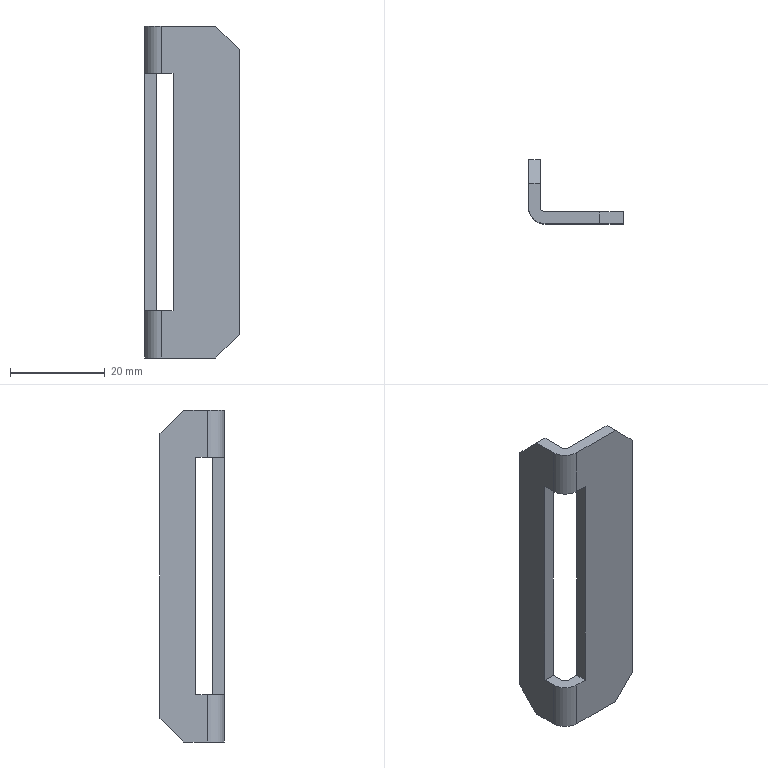Part | STEP file | AP0_JYDM_SHEET_15 | 1 solid | 20 faces | box 20 x 13.5 x 70 mm | volume 4064 mm3 | plane 16 | cylinder 4 | commonest cylinder face diameters 2 x2 7 x2
STEP:
#1=CARTESIAN_POINT('',(6.,2.5,25.));
#2=VERTEX_POINT('',#1);
#3=CARTESIAN_POINT('',(6.,2.5,-25.));
#4=VERTEX_POINT('',#3);
#5=CARTESIAN_POINT('',(6.,2.5,-35.));
#6=DIRECTION('',(0.,0.,-1.));
#7=VECTOR('',#6,1000.);
#8=LINE('',#5,#7);
#9=EDGE_CURVE('',#2,#4,#8,.T.);
#10=ORIENTED_EDGE('',*,*,#9,.F.);
#11=CARTESIAN_POINT('',(3.5,2.5,25.));
#12=VERTEX_POINT('',#11);
#13=CARTESIAN_POINT('',(0.,2.5,25.));
#14=DIRECTION('',(1.,0.,0.));
#15=VECTOR('',#14,1000.);
#16=LINE('',#13,#15);
#17=EDGE_CURVE('',#12,#2,#16,.T.);
#18=ORIENTED_EDGE('',*,*,#17,.F.);
#19=CARTESIAN_POINT('',(3.5,2.5,35.));
#20=VERTEX_POINT('',#19);
#21=CARTESIAN_POINT('',(3.5,2.5,-35.));
#22=DIRECTION('',(0.,0.,-1.));
#23=VECTOR('',#22,1000.);
#24=LINE('',#21,#23);
#25=EDGE_CURVE('',#20,#12,#24,.T.);
#26=ORIENTED_EDGE('',*,*,#25,.F.);
#27=CARTESIAN_POINT('',(15.,2.5,35.));
#28=VERTEX_POINT('',#27);
#29=CARTESIAN_POINT('',(0.,2.5,35.));
#30=DIRECTION('',(-1.,0.,0.));
#31=VECTOR('',#30,1000.);
#32=LINE('',#29,#31);
#33=EDGE_CURVE('',#28,#20,#32,.T.);
#34=ORIENTED_EDGE('',*,*,#33,.F.);
#35=CARTESIAN_POINT('',(20.,2.5,30.));
#36=VERTEX_POINT('',#35);
#37=CARTESIAN_POINT('',(20.,2.5,30.));
#38=DIRECTION('',(-0.7071,0.,0.7071));
#39=VECTOR('',#38,1000.);
#40=LINE('',#37,#39);
#41=EDGE_CURVE('',#36,#28,#40,.T.);
#42=ORIENTED_EDGE('',*,*,#41,.F.);
#43=CARTESIAN_POINT('',(20.,2.5,-30.));
#44=VERTEX_POINT('',#43);
#45=CARTESIAN_POINT('',(20.,2.5,-35.));
#46=DIRECTION('',(0.,0.,1.));
#47=VECTOR('',#46,1000.);
#48=LINE('',#45,#47);
#49=EDGE_CURVE('',#44,#36,#48,.T.);
#50=ORIENTED_EDGE('',*,*,#49,.F.);
#51=CARTESIAN_POINT('',(15.,2.5,-35.));
#52=VERTEX_POINT('',#51);
#53=CARTESIAN_POINT('',(15.,2.5,-35.));
#54=DIRECTION('',(0.7071,0.,0.7071));
#55=VECTOR('',#54,1000.);
#56=LINE('',#53,#55);
#57=EDGE_CURVE('',#52,#44,#56,.T.);
#58=ORIENTED_EDGE('',*,*,#57,.F.);
#59=CARTESIAN_POINT('',(3.5,2.5,-35.));
#60=VERTEX_POINT('',#59);
#61=CARTESIAN_POINT('',(0.,2.5,-35.));
#62=DIRECTION('',(1.,0.,0.));
#63=VECTOR('',#62,1000.);
#64=LINE('',#61,#63);
#65=EDGE_CURVE('',#60,#52,#64,.T.);
#66=ORIENTED_EDGE('',*,*,#65,.F.);
#67=CARTESIAN_POINT('',(3.5,2.5,-25.));
#68=VERTEX_POINT('',#67);
#69=CARTESIAN_POINT('',(3.5,2.5,-35.));
#70=DIRECTION('',(0.,0.,-1.));
#71=VECTOR('',#70,1000.);
#72=LINE('',#69,#71);
#73=EDGE_CURVE('',#68,#60,#72,.T.);
#74=ORIENTED_EDGE('',*,*,#73,.F.);
#75=CARTESIAN_POINT('',(0.,2.5,-25.));
#76=DIRECTION('',(-1.,0.,0.));
#77=VECTOR('',#76,1000.);
#78=LINE('',#75,#77);
#79=EDGE_CURVE('',#4,#68,#78,.T.);
#80=ORIENTED_EDGE('',*,*,#79,.F.);
#81=EDGE_LOOP('',(#10,#18,#26,#34,#42,#50,#58,#66,#74,#80));
#82=FACE_OUTER_BOUND('',#81,.T.);
#83=CARTESIAN_POINT('',(0.,2.5,-35.));
#84=DIRECTION('',(0.,-1.,0.));
#85=DIRECTION('',(0.,0.,-1.));
#86=AXIS2_PLACEMENT_3D('',#83,#84,#85);
#87=PLANE('',#86);
#88=ADVANCED_FACE('',(#82),#87,.F.);
#89=CARTESIAN_POINT('',(2.5,6.,-25.));
#90=VERTEX_POINT('',#89);
#91=CARTESIAN_POINT('',(2.5,3.5,-25.));
#92=VERTEX_POINT('',#91);
#93=CARTESIAN_POINT('',(2.5,1.25,-25.));
#94=DIRECTION('',(0.,-1.,0.));
#95=VECTOR('',#94,1000.);
#96=LINE('',#93,#95);
#97=EDGE_CURVE('',#90,#92,#96,.T.);
#98=ORIENTED_EDGE('',*,*,#97,.F.);
#99=CARTESIAN_POINT('',(0.,6.,-25.));
#100=VERTEX_POINT('',#99);
#101=CARTESIAN_POINT('',(4.75,6.,-25.));
#102=DIRECTION('',(1.,0.,0.));
#103=VECTOR('',#102,1000.);
#104=LINE('',#101,#103);
#105=EDGE_CURVE('',#100,#90,#104,.T.);
#106=ORIENTED_EDGE('',*,*,#105,.F.);
#107=CARTESIAN_POINT('',(0.,3.5,-25.));
#108=VERTEX_POINT('',#107);
#109=CARTESIAN_POINT('',(0.,1.25,-25.));
#110=DIRECTION('',(0.,1.,0.));
#111=VECTOR('',#110,1000.);
#112=LINE('',#109,#111);
#113=EDGE_CURVE('',#108,#100,#112,.T.);
#114=ORIENTED_EDGE('',*,*,#113,.F.);
#115=CARTESIAN_POINT('',(3.5,0.,-25.));
#116=VERTEX_POINT('',#115);
#117=CARTESIAN_POINT('',(3.5,3.5,-25.));
#118=DIRECTION('',(0.,0.,-1.));
#119=DIRECTION('',(-1.,0.,0.));
#120=AXIS2_PLACEMENT_3D('',#117,#118,#119);
#121=CIRCLE('',#120,3.5);
#122=EDGE_CURVE('',#116,#108,#121,.T.);
#123=ORIENTED_EDGE('',*,*,#122,.F.);
#124=CARTESIAN_POINT('',(6.,0.,-25.));
#125=VERTEX_POINT('',#124);
#126=CARTESIAN_POINT('',(4.75,0.,-25.));
#127=DIRECTION('',(-1.,0.,0.));
#128=VECTOR('',#127,1000.);
#129=LINE('',#126,#128);
#130=EDGE_CURVE('',#125,#116,#129,.T.);
#131=ORIENTED_EDGE('',*,*,#130,.F.);
#132=CARTESIAN_POINT('',(6.,1.25,-25.));
#133=DIRECTION('',(0.,-1.,0.));
#134=VECTOR('',#133,1000.);
#135=LINE('',#132,#134);
#136=EDGE_CURVE('',#4,#125,#135,.T.);
#137=ORIENTED_EDGE('',*,*,#136,.F.);
#138=ORIENTED_EDGE('',*,*,#79,.T.);
#139=CARTESIAN_POINT('',(3.5,3.5,-25.));
#140=DIRECTION('',(0.,0.,1.));
#141=DIRECTION('',(-1.,0.,0.));
#142=AXIS2_PLACEMENT_3D('',#139,#140,#141);
#143=CIRCLE('',#142,1.);
#144=EDGE_CURVE('',#92,#68,#143,.T.);
#145=ORIENTED_EDGE('',*,*,#144,.F.);
#146=EDGE_LOOP('',(#98,#106,#114,#123,#131,#137,#138,#145));
#147=FACE_OUTER_BOUND('',#146,.T.);
#148=CARTESIAN_POINT('',(4.75,1.25,-25.));
#149=DIRECTION('',(0.,0.,-1.));
#150=DIRECTION('',(-1.,0.,0.));
#151=AXIS2_PLACEMENT_3D('',#148,#149,#150);
#152=PLANE('',#151);
#153=ADVANCED_FACE('',(#147),#152,.F.);
#154=CARTESIAN_POINT('',(6.,0.,25.));
#155=VERTEX_POINT('',#154);
#156=CARTESIAN_POINT('',(6.,0.,0.));
#157=DIRECTION('',(0.,0.,-1.));
#158=VECTOR('',#157,1000.);
#159=LINE('',#156,#158);
#160=EDGE_CURVE('',#155,#125,#159,.T.);
#161=ORIENTED_EDGE('',*,*,#160,.F.);
#162=CARTESIAN_POINT('',(6.,1.25,25.));
#163=DIRECTION('',(0.,-1.,0.));
#164=VECTOR('',#163,1000.);
#165=LINE('',#162,#164);
#166=EDGE_CURVE('',#2,#155,#165,.T.);
#167=ORIENTED_EDGE('',*,*,#166,.F.);
#168=ORIENTED_EDGE('',*,*,#9,.T.);
#169=ORIENTED_EDGE('',*,*,#136,.T.);
#170=EDGE_LOOP('',(#161,#167,#168,#169));
#171=FACE_OUTER_BOUND('',#170,.T.);
#172=CARTESIAN_POINT('',(6.,1.25,0.));
#173=DIRECTION('',(1.,0.,0.));
#174=DIRECTION('',(0.,0.,-1.));
#175=AXIS2_PLACEMENT_3D('',#172,#173,#174);
#176=PLANE('',#175);
#177=ADVANCED_FACE('',(#171),#176,.F.);
#178=CARTESIAN_POINT('',(0.,6.,25.));
#179=VERTEX_POINT('',#178);
#180=CARTESIAN_POINT('',(2.5,6.,25.));
#181=VERTEX_POINT('',#180);
#182=CARTESIAN_POINT('',(4.75,6.,25.));
#183=DIRECTION('',(1.,0.,0.));
#184=VECTOR('',#183,1000.);
#185=LINE('',#182,#184);
#186=EDGE_CURVE('',#179,#181,#185,.T.);
#187=ORIENTED_EDGE('',*,*,#186,.T.);
#188=CARTESIAN_POINT('',(2.5,3.5,25.));
#189=VERTEX_POINT('',#188);
#190=CARTESIAN_POINT('',(2.5,1.25,25.));
#191=DIRECTION('',(0.,-1.,0.));
#192=VECTOR('',#191,1000.);
#193=LINE('',#190,#192);
#194=EDGE_CURVE('',#181,#189,#193,.T.);
#195=ORIENTED_EDGE('',*,*,#194,.T.);
#196=CARTESIAN_POINT('',(3.5,3.5,25.));
#197=DIRECTION('',(0.,0.,1.));
#198=DIRECTION('',(-1.,0.,0.));
#199=AXIS2_PLACEMENT_3D('',#196,#197,#198);
#200=CIRCLE('',#199,1.);
#201=EDGE_CURVE('',#189,#12,#200,.T.);
#202=ORIENTED_EDGE('',*,*,#201,.T.);
#203=ORIENTED_EDGE('',*,*,#17,.T.);
#204=ORIENTED_EDGE('',*,*,#166,.T.);
#205=CARTESIAN_POINT('',(3.5,0.,25.));
#206=VERTEX_POINT('',#205);
#207=CARTESIAN_POINT('',(4.75,0.,25.));
#208=DIRECTION('',(-1.,0.,0.));
#209=VECTOR('',#208,1000.);
#210=LINE('',#207,#209);
#211=EDGE_CURVE('',#155,#206,#210,.T.);
#212=ORIENTED_EDGE('',*,*,#211,.T.);
#213=CARTESIAN_POINT('',(0.,3.5,25.));
#214=VERTEX_POINT('',#213);
#215=CARTESIAN_POINT('',(3.5,3.5,25.));
#216=DIRECTION('',(0.,0.,-1.));
#217=DIRECTION('',(-1.,0.,0.));
#218=AXIS2_PLACEMENT_3D('',#215,#216,#217);
#219=CIRCLE('',#218,3.5);
#220=EDGE_CURVE('',#206,#214,#219,.T.);
#221=ORIENTED_EDGE('',*,*,#220,.T.);
#222=CARTESIAN_POINT('',(0.,1.25,25.));
#223=DIRECTION('',(0.,1.,0.));
#224=VECTOR('',#223,1000.);
#225=LINE('',#222,#224);
#226=EDGE_CURVE('',#214,#179,#225,.T.);
#227=ORIENTED_EDGE('',*,*,#226,.T.);
#228=EDGE_LOOP('',(#187,#195,#202,#203,#204,#212,#221,#227));
#229=FACE_OUTER_BOUND('',#228,.T.);
#230=CARTESIAN_POINT('',(4.75,1.25,25.));
#231=DIRECTION('',(0.,0.,-1.));
#232=DIRECTION('',(-1.,0.,0.));
#233=AXIS2_PLACEMENT_3D('',#230,#231,#232);
#234=PLANE('',#233);
#235=ADVANCED_FACE('',(#229),#234,.T.);
#236=ORIENTED_EDGE('',*,*,#201,.F.);
#237=CARTESIAN_POINT('',(2.5,3.5,35.));
#238=VERTEX_POINT('',#237);
#239=CARTESIAN_POINT('',(2.5,3.5,-35.));
#240=DIRECTION('',(0.,0.,-1.));
#241=VECTOR('',#240,1000.);
#242=LINE('',#239,#241);
#243=EDGE_CURVE('',#238,#189,#242,.T.);
#244=ORIENTED_EDGE('',*,*,#243,.F.);
#245=CARTESIAN_POINT('',(3.5,3.5,35.));
#246=DIRECTION('',(0.,0.,-1.));
#247=DIRECTION('',(-1.,0.,0.));
#248=AXIS2_PLACEMENT_3D('',#245,#246,#247);
#249=CIRCLE('',#248,1.);
#250=EDGE_CURVE('',#20,#238,#249,.T.);
#251=ORIENTED_EDGE('',*,*,#250,.F.);
#252=ORIENTED_EDGE('',*,*,#25,.T.);
#253=EDGE_LOOP('',(#236,#244,#251,#252));
#254=FACE_OUTER_BOUND('',#253,.T.);
#255=CARTESIAN_POINT('',(3.5,3.5,-35.));
#256=DIRECTION('',(0.,0.,-1.));
#257=DIRECTION('',(-1.,0.,0.));
#258=AXIS2_PLACEMENT_3D('',#255,#256,#257);
#259=CYLINDRICAL_SURFACE('',#258,1.);
#260=ADVANCED_FACE('',(#254),#259,.F.);
#261=CARTESIAN_POINT('',(2.5,8.5,35.));
#262=VERTEX_POINT('',#261);
#263=CARTESIAN_POINT('',(2.5,1.25,35.));
#264=DIRECTION('',(0.,-1.,0.));
#265=VECTOR('',#264,1000.);
#266=LINE('',#263,#265);
#267=EDGE_CURVE('',#262,#238,#266,.T.);
#268=ORIENTED_EDGE('',*,*,#267,.F.);
#269=CARTESIAN_POINT('',(0.,8.5,35.));
#270=VERTEX_POINT('',#269);
#271=CARTESIAN_POINT('',(11.75,8.5,35.));
#272=DIRECTION('',(1.,0.,0.));
#273=VECTOR('',#272,1000.);
#274=LINE('',#271,#273);
#275=EDGE_CURVE('',#270,#262,#274,.T.);
#276=ORIENTED_EDGE('',*,*,#275,.F.);
#277=CARTESIAN_POINT('',(0.,3.5,35.));
#278=VERTEX_POINT('',#277);
#279=CARTESIAN_POINT('',(0.,1.25,35.));
#280=DIRECTION('',(0.,1.,0.));
#281=VECTOR('',#280,1000.);
#282=LINE('',#279,#281);
#283=EDGE_CURVE('',#278,#270,#282,.T.);
#284=ORIENTED_EDGE('',*,*,#283,.F.);
#285=CARTESIAN_POINT('',(3.5,0.,35.));
#286=VERTEX_POINT('',#285);
#287=CARTESIAN_POINT('',(3.5,3.5,35.));
#288=DIRECTION('',(0.,0.,-1.));
#289=DIRECTION('',(-1.,0.,0.));
#290=AXIS2_PLACEMENT_3D('',#287,#288,#289);
#291=CIRCLE('',#290,3.5);
#292=EDGE_CURVE('',#286,#278,#291,.T.);
#293=ORIENTED_EDGE('',*,*,#292,.F.);
#294=CARTESIAN_POINT('',(15.,0.,35.));
#295=VERTEX_POINT('',#294);
#296=CARTESIAN_POINT('',(11.75,0.,35.));
#297=DIRECTION('',(-1.,0.,0.));
#298=VECTOR('',#297,1000.);
#299=LINE('',#296,#298);
#300=EDGE_CURVE('',#295,#286,#299,.T.);
#301=ORIENTED_EDGE('',*,*,#300,.F.);
#302=CARTESIAN_POINT('',(15.,1.25,35.));
#303=DIRECTION('',(0.,-1.,0.));
#304=VECTOR('',#303,1000.);
#305=LINE('',#302,#304);
#306=EDGE_CURVE('',#28,#295,#305,.T.);
#307=ORIENTED_EDGE('',*,*,#306,.F.);
#308=ORIENTED_EDGE('',*,*,#33,.T.);
#309=ORIENTED_EDGE('',*,*,#250,.T.);
#310=EDGE_LOOP('',(#268,#276,#284,#293,#301,#307,#308,#309));
#311=FACE_OUTER_BOUND('',#310,.T.);
#312=CARTESIAN_POINT('',(11.75,1.25,35.));
#313=DIRECTION('',(0.,0.,-1.));
#314=DIRECTION('',(-1.,0.,0.));
#315=AXIS2_PLACEMENT_3D('',#312,#313,#314);
#316=PLANE('',#315);
#317=ADVANCED_FACE('',(#311),#316,.F.);
#318=ORIENTED_EDGE('',*,*,#306,.T.);
#319=CARTESIAN_POINT('',(20.,0.,30.));
#320=VERTEX_POINT('',#319);
#321=CARTESIAN_POINT('',(17.5,0.,32.5));
#322=DIRECTION('',(0.7071,0.,-0.7071));
#323=VECTOR('',#322,1000.);
#324=LINE('',#321,#323);
#325=EDGE_CURVE('',#295,#320,#324,.T.);
#326=ORIENTED_EDGE('',*,*,#325,.T.);
#327=CARTESIAN_POINT('',(20.,1.25,30.));
#328=DIRECTION('',(0.,1.,0.));
#329=VECTOR('',#328,1000.);
#330=LINE('',#327,#329);
#331=EDGE_CURVE('',#320,#36,#330,.T.);
#332=ORIENTED_EDGE('',*,*,#331,.T.);
#333=ORIENTED_EDGE('',*,*,#41,.T.);
#334=EDGE_LOOP('',(#318,#326,#332,#333));
#335=FACE_OUTER_BOUND('',#334,.T.);
#336=CARTESIAN_POINT('',(17.5,1.25,32.5));
#337=DIRECTION('',(0.7071,0.,0.7071));
#338=DIRECTION('',(0.7071,0.,-0.7071));
#339=AXIS2_PLACEMENT_3D('',#336,#337,#338);
#340=PLANE('',#339);
#341=ADVANCED_FACE('',(#335),#340,.T.);
#342=CARTESIAN_POINT('',(20.,0.,-30.));
#343=VERTEX_POINT('',#342);
#344=CARTESIAN_POINT('',(20.,0.,0.));
#345=DIRECTION('',(0.,0.,-1.));
#346=VECTOR('',#345,1000.);
#347=LINE('',#344,#346);
#348=EDGE_CURVE('',#320,#343,#347,.T.);
#349=ORIENTED_EDGE('',*,*,#348,.T.);
#350=CARTESIAN_POINT('',(20.,1.25,-30.));
#351=DIRECTION('',(0.,1.,0.));
#352=VECTOR('',#351,1000.);
#353=LINE('',#350,#352);
#354=EDGE_CURVE('',#343,#44,#353,.T.);
#355=ORIENTED_EDGE('',*,*,#354,.T.);
#356=ORIENTED_EDGE('',*,*,#49,.T.);
#357=ORIENTED_EDGE('',*,*,#331,.F.);
#358=EDGE_LOOP('',(#349,#355,#356,#357));
#359=FACE_OUTER_BOUND('',#358,.T.);
#360=CARTESIAN_POINT('',(20.,1.25,0.));
#361=DIRECTION('',(1.,0.,0.));
#362=DIRECTION('',(0.,0.,-1.));
#363=AXIS2_PLACEMENT_3D('',#360,#361,#362);
#364=PLANE('',#363);
#365=ADVANCED_FACE('',(#359),#364,.T.);
#366=ORIENTED_EDGE('',*,*,#354,.F.);
#367=CARTESIAN_POINT('',(15.,0.,-35.));
#368=VERTEX_POINT('',#367);
#369=CARTESIAN_POINT('',(17.5,0.,-32.5));
#370=DIRECTION('',(-0.7071,0.,-0.7071));
#371=VECTOR('',#370,1000.);
#372=LINE('',#369,#371);
#373=EDGE_CURVE('',#343,#368,#372,.T.);
#374=ORIENTED_EDGE('',*,*,#373,.T.);
#375=CARTESIAN_POINT('',(15.,1.25,-35.));
#376=DIRECTION('',(0.,1.,0.));
#377=VECTOR('',#376,1000.);
#378=LINE('',#375,#377);
#379=EDGE_CURVE('',#368,#52,#378,.T.);
#380=ORIENTED_EDGE('',*,*,#379,.T.);
#381=ORIENTED_EDGE('',*,*,#57,.T.);
#382=EDGE_LOOP('',(#366,#374,#380,#381));
#383=FACE_OUTER_BOUND('',#382,.T.);
#384=CARTESIAN_POINT('',(17.5,1.25,-32.5));
#385=DIRECTION('',(0.7071,0.,-0.7071));
#386=DIRECTION('',(-0.7071,0.,-0.7071));
#387=AXIS2_PLACEMENT_3D('',#384,#385,#386);
#388=PLANE('',#387);
#389=ADVANCED_FACE('',(#383),#388,.T.);
#390=CARTESIAN_POINT('',(0.,3.5,-35.));
#391=VERTEX_POINT('',#390);
#392=CARTESIAN_POINT('',(0.,8.5,-35.));
#393=VERTEX_POINT('',#392);
#394=CARTESIAN_POINT('',(0.,1.25,-35.));
#395=DIRECTION('',(0.,1.,0.));
#396=VECTOR('',#395,1000.);
#397=LINE('',#394,#396);
#398=EDGE_CURVE('',#391,#393,#397,.T.);
#399=ORIENTED_EDGE('',*,*,#398,.T.);
#400=CARTESIAN_POINT('',(2.5,8.5,-35.));
#401=VERTEX_POINT('',#400);
#402=CARTESIAN_POINT('',(11.75,8.5,-35.));
#403=DIRECTION('',(1.,0.,0.));
#404=VECTOR('',#403,1000.);
#405=LINE('',#402,#404);
#406=EDGE_CURVE('',#393,#401,#405,.T.);
#407=ORIENTED_EDGE('',*,*,#406,.T.);
#408=CARTESIAN_POINT('',(2.5,3.5,-35.));
#409=VERTEX_POINT('',#408);
#410=CARTESIAN_POINT('',(2.5,1.25,-35.));
#411=DIRECTION('',(0.,-1.,0.));
#412=VECTOR('',#411,1000.);
#413=LINE('',#410,#412);
#414=EDGE_CURVE('',#401,#409,#413,.T.);
#415=ORIENTED_EDGE('',*,*,#414,.T.);
#416=CARTESIAN_POINT('',(3.5,3.5,-35.));
#417=DIRECTION('',(0.,0.,1.));
#418=DIRECTION('',(-1.,0.,0.));
#419=AXIS2_PLACEMENT_3D('',#416,#417,#418);
#420=CIRCLE('',#419,1.);
#421=EDGE_CURVE('',#409,#60,#420,.T.);
#422=ORIENTED_EDGE('',*,*,#421,.T.);
#423=ORIENTED_EDGE('',*,*,#65,.T.);
#424=ORIENTED_EDGE('',*,*,#379,.F.);
#425=CARTESIAN_POINT('',(3.5,0.,-35.));
#426=VERTEX_POINT('',#425);
#427=CARTESIAN_POINT('',(11.75,0.,-35.));
#428=DIRECTION('',(-1.,0.,0.));
#429=VECTOR('',#428,1000.);
#430=LINE('',#427,#429);
#431=EDGE_CURVE('',#368,#426,#430,.T.);
#432=ORIENTED_EDGE('',*,*,#431,.T.);
#433=CARTESIAN_POINT('',(3.5,3.5,-35.));
#434=DIRECTION('',(0.,0.,-1.));
#435=DIRECTION('',(-1.,0.,0.));
#436=AXIS2_PLACEMENT_3D('',#433,#434,#435);
#437=CIRCLE('',#436,3.5);
#438=EDGE_CURVE('',#426,#391,#437,.T.);
#439=ORIENTED_EDGE('',*,*,#438,.T.);
#440=EDGE_LOOP('',(#399,#407,#415,#422,#423,#424,#432,#439));
#441=FACE_OUTER_BOUND('',#440,.T.);
#442=CARTESIAN_POINT('',(11.75,1.25,-35.));
#443=DIRECTION('',(0.,0.,-1.));
#444=DIRECTION('',(-1.,0.,0.));
#445=AXIS2_PLACEMENT_3D('',#442,#443,#444);
#446=PLANE('',#445);
#447=ADVANCED_FACE('',(#441),#446,.T.);
#448=ORIENTED_EDGE('',*,*,#144,.T.);
#449=ORIENTED_EDGE('',*,*,#73,.T.);
#450=ORIENTED_EDGE('',*,*,#421,.F.);
#451=CARTESIAN_POINT('',(2.5,3.5,-35.));
#452=DIRECTION('',(0.,0.,-1.));
#453=VECTOR('',#452,1000.);
#454=LINE('',#451,#453);
#455=EDGE_CURVE('',#92,#409,#454,.T.);
#456=ORIENTED_EDGE('',*,*,#455,.F.);
#457=EDGE_LOOP('',(#448,#449,#450,#456));
#458=FACE_OUTER_BOUND('',#457,.T.);
#459=CARTESIAN_POINT('',(3.5,3.5,-35.));
#460=DIRECTION('',(0.,0.,-1.));
#461=DIRECTION('',(-1.,0.,0.));
#462=AXIS2_PLACEMENT_3D('',#459,#460,#461);
#463=CYLINDRICAL_SURFACE('',#462,1.);
#464=ADVANCED_FACE('',(#458),#463,.F.);
#465=CARTESIAN_POINT('',(2.5,6.,-35.));
#466=DIRECTION('',(0.,0.,1.));
#467=VECTOR('',#466,1000.);
#468=LINE('',#465,#467);
#469=EDGE_CURVE('',#90,#181,#468,.T.);
#470=ORIENTED_EDGE('',*,*,#469,.F.);
#471=ORIENTED_EDGE('',*,*,#97,.T.);
#472=ORIENTED_EDGE('',*,*,#455,.T.);
#473=ORIENTED_EDGE('',*,*,#414,.F.);
#474=CARTESIAN_POINT('',(2.5,13.5,-30.));
#475=VERTEX_POINT('',#474);
#476=CARTESIAN_POINT('',(2.5,13.5,-30.));
#477=DIRECTION('',(0.,-0.7071,-0.7071));
#478=VECTOR('',#477,1000.);
#479=LINE('',#476,#478);
#480=EDGE_CURVE('',#475,#401,#479,.T.);
#481=ORIENTED_EDGE('',*,*,#480,.F.);
#482=CARTESIAN_POINT('',(2.5,13.5,30.));
#483=VERTEX_POINT('',#482);
#484=CARTESIAN_POINT('',(2.5,13.5,-35.));
#485=DIRECTION('',(0.,0.,-1.));
#486=VECTOR('',#485,1000.);
#487=LINE('',#484,#486);
#488=EDGE_CURVE('',#483,#475,#487,.T.);
#489=ORIENTED_EDGE('',*,*,#488,.F.);
#490=CARTESIAN_POINT('',(2.5,8.5,35.));
#491=DIRECTION('',(0.,0.7071,-0.7071));
#492=VECTOR('',#491,1000.);
#493=LINE('',#490,#492);
#494=EDGE_CURVE('',#262,#483,#493,.T.);
#495=ORIENTED_EDGE('',*,*,#494,.F.);
#496=ORIENTED_EDGE('',*,*,#267,.T.);
#497=ORIENTED_EDGE('',*,*,#243,.T.);
#498=ORIENTED_EDGE('',*,*,#194,.F.);
#499=EDGE_LOOP('',(#470,#471,#472,#473,#481,#489,#495,#496,#497,#498));
#500=FACE_OUTER_BOUND('',#499,.T.);
#501=CARTESIAN_POINT('',(2.5,13.5,-35.));
#502=DIRECTION('',(-1.,0.,0.));
#503=DIRECTION('',(0.,0.,1.));
#504=AXIS2_PLACEMENT_3D('',#501,#502,#503);
#505=PLANE('',#504);
#506=ADVANCED_FACE('',(#500),#505,.F.);
#507=ORIENTED_EDGE('',*,*,#186,.F.);
#508=CARTESIAN_POINT('',(0.,6.,0.));
#509=DIRECTION('',(0.,0.,-1.));
#510=VECTOR('',#509,1000.);
#511=LINE('',#508,#510);
#512=EDGE_CURVE('',#179,#100,#511,.T.);
#513=ORIENTED_EDGE('',*,*,#512,.T.);
#514=ORIENTED_EDGE('',*,*,#105,.T.);
#515=ORIENTED_EDGE('',*,*,#469,.T.);
#516=EDGE_LOOP('',(#507,#513,#514,#515));
#517=FACE_OUTER_BOUND('',#516,.T.);
#518=CARTESIAN_POINT('',(1.25,6.,0.));
#519=DIRECTION('',(0.,-1.,0.));
#520=DIRECTION('',(0.,0.,-1.));
#521=AXIS2_PLACEMENT_3D('',#518,#519,#520);
#522=PLANE('',#521);
#523=ADVANCED_FACE('',(#517),#522,.T.);
#524=ORIENTED_EDGE('',*,*,#113,.T.);
#525=ORIENTED_EDGE('',*,*,#512,.F.);
#526=ORIENTED_EDGE('',*,*,#226,.F.);
#527=CARTESIAN_POINT('',(0.,3.5,-35.));
#528=DIRECTION('',(0.,0.,1.));
#529=VECTOR('',#528,1000.);
#530=LINE('',#527,#529);
#531=EDGE_CURVE('',#214,#278,#530,.T.);
#532=ORIENTED_EDGE('',*,*,#531,.T.);
#533=ORIENTED_EDGE('',*,*,#283,.T.);
#534=CARTESIAN_POINT('',(0.,13.5,30.));
#535=VERTEX_POINT('',#534);
#536=CARTESIAN_POINT('',(0.,8.5,35.));
#537=DIRECTION('',(0.,0.7071,-0.7071));
#538=VECTOR('',#537,1000.);
#539=LINE('',#536,#538);
#540=EDGE_CURVE('',#270,#535,#539,.T.);
#541=ORIENTED_EDGE('',*,*,#540,.T.);
#542=CARTESIAN_POINT('',(0.,13.5,-30.));
#543=VERTEX_POINT('',#542);
#544=CARTESIAN_POINT('',(0.,13.5,-35.));
#545=DIRECTION('',(0.,0.,-1.));
#546=VECTOR('',#545,1000.);
#547=LINE('',#544,#546);
#548=EDGE_CURVE('',#535,#543,#547,.T.);
#549=ORIENTED_EDGE('',*,*,#548,.T.);
#550=CARTESIAN_POINT('',(0.,13.5,-30.));
#551=DIRECTION('',(0.,-0.7071,-0.7071));
#552=VECTOR('',#551,1000.);
#553=LINE('',#550,#552);
#554=EDGE_CURVE('',#543,#393,#553,.T.);
#555=ORIENTED_EDGE('',*,*,#554,.T.);
#556=ORIENTED_EDGE('',*,*,#398,.F.);
#557=CARTESIAN_POINT('',(0.,3.5,-35.));
#558=DIRECTION('',(0.,0.,1.));
#559=VECTOR('',#558,1000.);
#560=LINE('',#557,#559);
#561=EDGE_CURVE('',#391,#108,#560,.T.);
#562=ORIENTED_EDGE('',*,*,#561,.T.);
#563=EDGE_LOOP('',(#524,#525,#526,#532,#533,#541,#549,#555,#556,#562));
#564=FACE_OUTER_BOUND('',#563,.T.);
#565=CARTESIAN_POINT('',(0.,13.5,-35.));
#566=DIRECTION('',(-1.,0.,0.));
#567=DIRECTION('',(0.,0.,1.));
#568=AXIS2_PLACEMENT_3D('',#565,#566,#567);
#569=PLANE('',#568);
#570=ADVANCED_FACE('',(#564),#569,.T.);
#571=CARTESIAN_POINT('',(3.5,0.,-35.));
#572=DIRECTION('',(0.,0.,1.));
#573=VECTOR('',#572,1000.);
#574=LINE('',#571,#573);
#575=EDGE_CURVE('',#426,#116,#574,.T.);
#576=ORIENTED_EDGE('',*,*,#575,.T.);
#577=ORIENTED_EDGE('',*,*,#122,.T.);
#578=ORIENTED_EDGE('',*,*,#561,.F.);
#579=ORIENTED_EDGE('',*,*,#438,.F.);
#580=EDGE_LOOP('',(#576,#577,#578,#579));
#581=FACE_OUTER_BOUND('',#580,.T.);
#582=CARTESIAN_POINT('',(3.5,3.5,-35.));
#583=DIRECTION('',(0.,0.,-1.));
#584=DIRECTION('',(-1.,0.,0.));
#585=AXIS2_PLACEMENT_3D('',#582,#583,#584);
#586=CYLINDRICAL_SURFACE('',#585,3.5);
#587=ADVANCED_FACE('',(#581),#586,.T.);
#588=ORIENTED_EDGE('',*,*,#211,.F.);
#589=ORIENTED_EDGE('',*,*,#160,.T.);
#590=ORIENTED_EDGE('',*,*,#130,.T.);
#591=ORIENTED_EDGE('',*,*,#575,.F.);
#592=ORIENTED_EDGE('',*,*,#431,.F.);
#593=ORIENTED_EDGE('',*,*,#373,.F.);
#594=ORIENTED_EDGE('',*,*,#348,.F.);
#595=ORIENTED_EDGE('',*,*,#325,.F.);
#596=ORIENTED_EDGE('',*,*,#300,.T.);
#597=CARTESIAN_POINT('',(3.5,0.,-35.));
#598=DIRECTION('',(0.,0.,-1.));
#599=VECTOR('',#598,1000.);
#600=LINE('',#597,#599);
#601=EDGE_CURVE('',#286,#206,#600,.T.);
#602=ORIENTED_EDGE('',*,*,#601,.T.);
#603=EDGE_LOOP('',(#588,#589,#590,#591,#592,#593,#594,#595,#596,#602));
#604=FACE_OUTER_BOUND('',#603,.T.);
#605=CARTESIAN_POINT('',(0.,0.,-35.));
#606=DIRECTION('',(0.,-1.,0.));
#607=DIRECTION('',(0.,0.,-1.));
#608=AXIS2_PLACEMENT_3D('',#605,#606,#607);
#609=PLANE('',#608);
#610=ADVANCED_FACE('',(#604),#609,.T.);
#611=ORIENTED_EDGE('',*,*,#531,.F.);
#612=ORIENTED_EDGE('',*,*,#220,.F.);
#613=ORIENTED_EDGE('',*,*,#601,.F.);
#614=ORIENTED_EDGE('',*,*,#292,.T.);
#615=EDGE_LOOP('',(#611,#612,#613,#614));
#616=FACE_OUTER_BOUND('',#615,.T.);
#617=CARTESIAN_POINT('',(3.5,3.5,-35.));
#618=DIRECTION('',(0.,0.,-1.));
#619=DIRECTION('',(-1.,0.,0.));
#620=AXIS2_PLACEMENT_3D('',#617,#618,#619);
#621=CYLINDRICAL_SURFACE('',#620,3.5);
#622=ADVANCED_FACE('',(#616),#621,.T.);
#623=CARTESIAN_POINT('',(1.25,13.5,30.));
#624=DIRECTION('',(-1.,0.,0.));
#625=VECTOR('',#624,1000.);
#626=LINE('',#623,#625);
#627=EDGE_CURVE('',#483,#535,#626,.T.);
#628=ORIENTED_EDGE('',*,*,#627,.T.);
#629=ORIENTED_EDGE('',*,*,#540,.F.);
#630=ORIENTED_EDGE('',*,*,#275,.T.);
#631=ORIENTED_EDGE('',*,*,#494,.T.);
#632=EDGE_LOOP('',(#628,#629,#630,#631));
#633=FACE_OUTER_BOUND('',#632,.T.);
#634=CARTESIAN_POINT('',(1.25,11.,32.5));
#635=DIRECTION('',(0.,0.7071,0.7071));
#636=DIRECTION('',(0.,-0.7071,0.7071));
#637=AXIS2_PLACEMENT_3D('',#634,#635,#636);
#638=PLANE('',#637);
#639=ADVANCED_FACE('',(#633),#638,.T.);
#640=ORIENTED_EDGE('',*,*,#406,.F.);
#641=ORIENTED_EDGE('',*,*,#554,.F.);
#642=CARTESIAN_POINT('',(1.25,13.5,-30.));
#643=DIRECTION('',(1.,0.,0.));
#644=VECTOR('',#643,1000.);
#645=LINE('',#642,#644);
#646=EDGE_CURVE('',#543,#475,#645,.T.);
#647=ORIENTED_EDGE('',*,*,#646,.T.);
#648=ORIENTED_EDGE('',*,*,#480,.T.);
#649=EDGE_LOOP('',(#640,#641,#647,#648));
#650=FACE_OUTER_BOUND('',#649,.T.);
#651=CARTESIAN_POINT('',(1.25,11.,-32.5));
#652=DIRECTION('',(0.,0.7071,-0.7071));
#653=DIRECTION('',(0.,0.7071,0.7071));
#654=AXIS2_PLACEMENT_3D('',#651,#652,#653);
#655=PLANE('',#654);
#656=ADVANCED_FACE('',(#650),#655,.T.);
#657=ORIENTED_EDGE('',*,*,#627,.F.);
#658=ORIENTED_EDGE('',*,*,#488,.T.);
#659=ORIENTED_EDGE('',*,*,#646,.F.);
#660=ORIENTED_EDGE('',*,*,#548,.F.);
#661=EDGE_LOOP('',(#657,#658,#659,#660));
#662=FACE_OUTER_BOUND('',#661,.T.);
#663=CARTESIAN_POINT('',(1.25,13.5,0.));
#664=DIRECTION('',(0.,-1.,0.));
#665=DIRECTION('',(0.,0.,-1.));
#666=AXIS2_PLACEMENT_3D('',#663,#664,#665);
#667=PLANE('',#666);
#668=ADVANCED_FACE('',(#662),#667,.F.);
#669=CLOSED_SHELL('',(#88,#153,#177,#235,#260,#317,#341,#365,#389,#447,#464,#506,#523,#570,#587,#610,#622,#639,#656,#668));
#670=MANIFOLD_SOLID_BREP('',#669);
#671=CARTESIAN_POINT('',(0.,0.,0.));
#672=DIRECTION('',(0.,0.,1.));
#673=DIRECTION('',(1.,0.,0.));
#674=AXIS2_PLACEMENT_3D('',#671,#672,#673);
#675=(LENGTH_UNIT()NAMED_UNIT(*)SI_UNIT(.MILLI.,.METRE.));
#676=UNCERTAINTY_MEASURE_WITH_UNIT(LENGTH_MEASURE(0.00001),#675,'','');
#677=(NAMED_UNIT(*)PLANE_ANGLE_UNIT()SI_UNIT($,.RADIAN.));
#678=(NAMED_UNIT(*)SI_UNIT($,.STERADIAN.)SOLID_ANGLE_UNIT());
#679=(GEOMETRIC_REPRESENTATION_CONTEXT(3)GLOBAL_UNCERTAINTY_ASSIGNED_CONTEXT((#676))GLOBAL_UNIT_ASSIGNED_CONTEXT((#675,#677,#678))REPRESENTATION_CONTEXT('',''));
#680=ADVANCED_BREP_SHAPE_REPRESENTATION('',(#670,#674),#679);